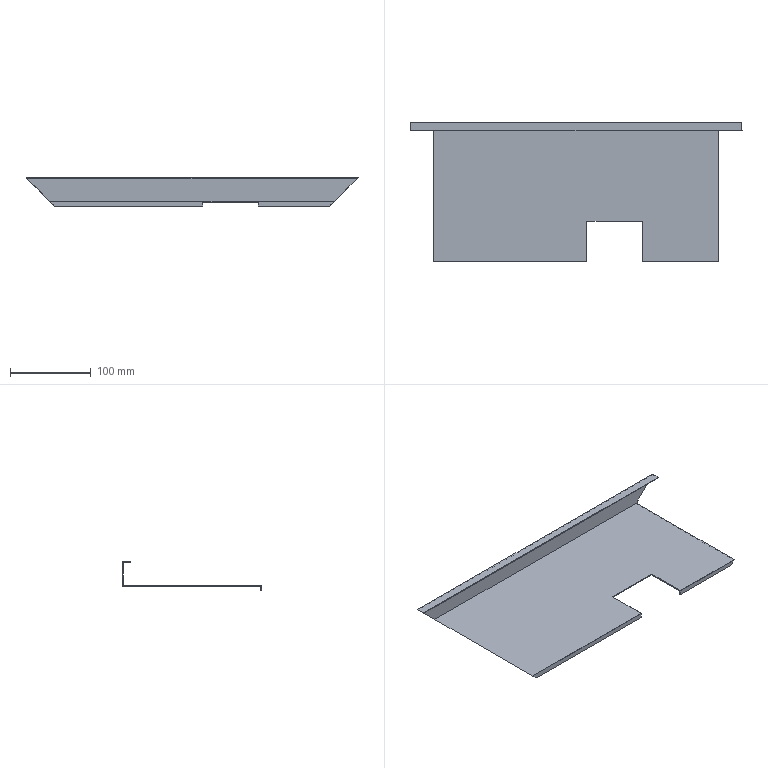Part | STEP file | 09-06 Inner side plate 3 | 1 solid | 18 faces | box 410 x 172 x 35 mm | volume 73059 mm3 | plane 18
STEP:
#1=CARTESIAN_POINT('',(0.,0.,0.));
#2=DIRECTION('',(0.,0.,1.));
#3=DIRECTION('',(1.,0.,0.));
#4=AXIS2_PLACEMENT_3D('',#1,#2,#3);
#5=CARTESIAN_POINT('',(381.,0.,1.));
#6=VERTEX_POINT('',#5);
#7=CARTESIAN_POINT('',(287.,0.,1.));
#8=VERTEX_POINT('',#7);
#9=CARTESIAN_POINT('',(205.,0.,1.));
#10=DIRECTION('',(-1.,0.,0.));
#11=VECTOR('',#10,1.);
#12=LINE('',#9,#11);
#13=CARTESIAN_POINT('',(29.,0.,1.));
#14=DIRECTION('',(0.,0.,-1.));
#15=DIRECTION('',(0.,1.,0.));
#16=AXIS2_PLACEMENT_3D('',#13,#14,#15);
#17=PLANE('',#16);
#18=CARTESIAN_POINT('',(0.,176.));
#19=DIRECTION('',(0.,-1.));
#20=VECTOR('',#19,1.);
#21=LINE('',#18,#20);
#22=(GEOMETRIC_REPRESENTATION_CONTEXT(2)PARAMETRIC_REPRESENTATION_CONTEXT()REPRESENTATION_CONTEXT('',''));
#23=DEFINITIONAL_REPRESENTATION('',(#21),#22);
#24=PCURVE('',#17,#23);
#25=CARTESIAN_POINT('',(287.,0.,-5.));
#26=DIRECTION('',(0.,1.,0.));
#27=DIRECTION('',(0.,0.,1.));
#28=AXIS2_PLACEMENT_3D('',#25,#26,#27);
#29=PLANE('',#28);
#30=CARTESIAN_POINT('',(6.,-82.));
#31=DIRECTION('',(0.,-1.));
#32=VECTOR('',#31,1.);
#33=LINE('',#30,#32);
#34=(GEOMETRIC_REPRESENTATION_CONTEXT(2)PARAMETRIC_REPRESENTATION_CONTEXT()REPRESENTATION_CONTEXT('',''));
#35=DEFINITIONAL_REPRESENTATION('',(#33),#34);
#36=PCURVE('',#29,#35);
#37=SURFACE_CURVE('',#12,(#24,#36),.PCURVE_S1.);
#38=EDGE_CURVE('',#6,#8,#37,.T.);
#39=ORIENTED_EDGE('',*,*,#38,.F.);
#40=CARTESIAN_POINT('',(381.,171.,1.));
#41=VERTEX_POINT('',#40);
#42=CARTESIAN_POINT('',(381.,85.5,1.));
#43=DIRECTION('',(0.,-1.,0.));
#44=VECTOR('',#43,1.);
#45=LINE('',#42,#44);
#46=CARTESIAN_POINT('',(85.5,352.));
#47=DIRECTION('',(-1.,0.));
#48=VECTOR('',#47,1.);
#49=LINE('',#46,#48);
#50=(GEOMETRIC_REPRESENTATION_CONTEXT(2)PARAMETRIC_REPRESENTATION_CONTEXT()REPRESENTATION_CONTEXT('',''));
#51=DEFINITIONAL_REPRESENTATION('',(#49),#50);
#52=PCURVE('',#17,#51);
#53=CARTESIAN_POINT('',(375.,0.,-5.));
#54=DIRECTION('',(-0.7071,0.,0.7071));
#55=DIRECTION('',(0.7071,0.,0.7071));
#56=AXIS2_PLACEMENT_3D('',#53,#54,#55);
#57=PLANE('',#56);
#58=CARTESIAN_POINT('',(8.485,85.5));
#59=DIRECTION('',(0.,-1.));
#60=VECTOR('',#59,1.);
#61=LINE('',#58,#60);
#62=(GEOMETRIC_REPRESENTATION_CONTEXT(2)PARAMETRIC_REPRESENTATION_CONTEXT()REPRESENTATION_CONTEXT('',''));
#63=DEFINITIONAL_REPRESENTATION('',(#61),#62);
#64=PCURVE('',#57,#63);
#65=SURFACE_CURVE('',#45,(#52,#64),.PCURVE_S1.);
#66=EDGE_CURVE('',#41,#6,#65,.T.);
#67=ORIENTED_EDGE('',*,*,#66,.F.);
#68=CARTESIAN_POINT('',(29.,171.,1.));
#69=VERTEX_POINT('',#68);
#70=CARTESIAN_POINT('',(205.,171.,1.));
#71=DIRECTION('',(1.,0.,0.));
#72=VECTOR('',#71,1.);
#73=LINE('',#70,#72);
#74=CARTESIAN_POINT('',(171.,176.));
#75=DIRECTION('',(0.,1.));
#76=VECTOR('',#75,1.);
#77=LINE('',#74,#76);
#78=(GEOMETRIC_REPRESENTATION_CONTEXT(2)PARAMETRIC_REPRESENTATION_CONTEXT()REPRESENTATION_CONTEXT('',''));
#79=DEFINITIONAL_REPRESENTATION('',(#77),#78);
#80=PCURVE('',#17,#79);
#81=CARTESIAN_POINT('',(-1.448,171.,1.));
#82=DIRECTION('',(0.,1.,0.));
#83=DIRECTION('',(0.,0.,1.));
#84=AXIS2_PLACEMENT_3D('',#81,#82,#83);
#85=PLANE('',#84);
#86=CARTESIAN_POINT('',(0.,206.448));
#87=DIRECTION('',(0.,1.));
#88=VECTOR('',#87,1.);
#89=LINE('',#86,#88);
#90=(GEOMETRIC_REPRESENTATION_CONTEXT(2)PARAMETRIC_REPRESENTATION_CONTEXT()REPRESENTATION_CONTEXT('',''));
#91=DEFINITIONAL_REPRESENTATION('',(#89),#90);
#92=PCURVE('',#85,#91);
#93=SURFACE_CURVE('',#73,(#80,#92),.PCURVE_S1.);
#94=EDGE_CURVE('',#69,#41,#93,.T.);
#95=ORIENTED_EDGE('',*,*,#94,.F.);
#96=CARTESIAN_POINT('',(29.,0.,1.));
#97=VERTEX_POINT('',#96);
#98=CARTESIAN_POINT('',(29.,85.5,1.));
#99=DIRECTION('',(0.,1.,0.));
#100=VECTOR('',#99,1.);
#101=LINE('',#98,#100);
#102=CARTESIAN_POINT('',(85.5,0.));
#103=DIRECTION('',(1.,0.));
#104=VECTOR('',#103,1.);
#105=LINE('',#102,#104);
#106=(GEOMETRIC_REPRESENTATION_CONTEXT(2)PARAMETRIC_REPRESENTATION_CONTEXT()REPRESENTATION_CONTEXT('',''));
#107=DEFINITIONAL_REPRESENTATION('',(#105),#106);
#108=PCURVE('',#17,#107);
#109=CARTESIAN_POINT('',(0.,0.,30.));
#110=DIRECTION('',(0.7071,0.,0.7071));
#111=DIRECTION('',(0.7071,0.,-0.7071));
#112=AXIS2_PLACEMENT_3D('',#109,#110,#111);
#113=PLANE('',#112);
#114=CARTESIAN_POINT('',(41.012,85.5));
#115=DIRECTION('',(0.,1.));
#116=VECTOR('',#115,1.);
#117=LINE('',#114,#116);
#118=(GEOMETRIC_REPRESENTATION_CONTEXT(2)PARAMETRIC_REPRESENTATION_CONTEXT()REPRESENTATION_CONTEXT('',''));
#119=DEFINITIONAL_REPRESENTATION('',(#117),#118);
#120=PCURVE('',#113,#119);
#121=SURFACE_CURVE('',#101,(#108,#120),.PCURVE_S1.);
#122=EDGE_CURVE('',#97,#69,#121,.T.);
#123=ORIENTED_EDGE('',*,*,#122,.F.);
#124=CARTESIAN_POINT('',(218.5,0.,1.));
#125=VERTEX_POINT('',#124);
#126=CARTESIAN_POINT('',(205.,0.,1.));
#127=DIRECTION('',(-1.,0.,0.));
#128=VECTOR('',#127,1.);
#129=LINE('',#126,#128);
#130=CARTESIAN_POINT('',(0.,176.));
#131=DIRECTION('',(0.,-1.));
#132=VECTOR('',#131,1.);
#133=LINE('',#130,#132);
#134=(GEOMETRIC_REPRESENTATION_CONTEXT(2)PARAMETRIC_REPRESENTATION_CONTEXT()REPRESENTATION_CONTEXT('',''));
#135=DEFINITIONAL_REPRESENTATION('',(#133),#134);
#136=PCURVE('',#17,#135);
#137=CARTESIAN_POINT('',(27.863,0.,-5.));
#138=DIRECTION('',(0.,1.,0.));
#139=DIRECTION('',(0.,0.,1.));
#140=AXIS2_PLACEMENT_3D('',#137,#138,#139);
#141=PLANE('',#140);
#142=CARTESIAN_POINT('',(6.,177.137));
#143=DIRECTION('',(0.,-1.));
#144=VECTOR('',#143,1.);
#145=LINE('',#142,#144);
#146=(GEOMETRIC_REPRESENTATION_CONTEXT(2)PARAMETRIC_REPRESENTATION_CONTEXT()REPRESENTATION_CONTEXT('',''));
#147=DEFINITIONAL_REPRESENTATION('',(#145),#146);
#148=PCURVE('',#141,#147);
#149=SURFACE_CURVE('',#129,(#136,#148),.PCURVE_S1.);
#150=EDGE_CURVE('',#125,#97,#149,.T.);
#151=ORIENTED_EDGE('',*,*,#150,.F.);
#152=CARTESIAN_POINT('',(218.5,50.,1.));
#153=VERTEX_POINT('',#152);
#154=CARTESIAN_POINT('',(218.5,85.5,1.));
#155=DIRECTION('',(0.,-1.,0.));
#156=VECTOR('',#155,1.);
#157=LINE('',#154,#156);
#158=CARTESIAN_POINT('',(85.5,189.5));
#159=DIRECTION('',(-1.,0.));
#160=VECTOR('',#159,1.);
#161=LINE('',#158,#160);
#162=(GEOMETRIC_REPRESENTATION_CONTEXT(2)PARAMETRIC_REPRESENTATION_CONTEXT()REPRESENTATION_CONTEXT('',''));
#163=DEFINITIONAL_REPRESENTATION('',(#161),#162);
#164=PCURVE('',#17,#163);
#165=CARTESIAN_POINT('',(218.5,0.,1.));
#166=DIRECTION('',(1.,0.,0.));
#167=DIRECTION('',(0.,0.,-1.));
#168=AXIS2_PLACEMENT_3D('',#165,#166,#167);
#169=PLANE('',#168);
#170=CARTESIAN_POINT('',(0.,85.5));
#171=DIRECTION('',(0.,-1.));
#172=VECTOR('',#171,1.);
#173=LINE('',#170,#172);
#174=(GEOMETRIC_REPRESENTATION_CONTEXT(2)PARAMETRIC_REPRESENTATION_CONTEXT()REPRESENTATION_CONTEXT('',''));
#175=DEFINITIONAL_REPRESENTATION('',(#173),#174);
#176=PCURVE('',#169,#175);
#177=SURFACE_CURVE('',#157,(#164,#176),.PCURVE_S1.);
#178=EDGE_CURVE('',#153,#125,#177,.T.);
#179=ORIENTED_EDGE('',*,*,#178,.F.);
#180=CARTESIAN_POINT('',(287.,50.,1.));
#181=VERTEX_POINT('',#180);
#182=CARTESIAN_POINT('',(205.,50.,1.));
#183=DIRECTION('',(-1.,0.,0.));
#184=VECTOR('',#183,1.);
#185=LINE('',#182,#184);
#186=CARTESIAN_POINT('',(50.,176.));
#187=DIRECTION('',(0.,-1.));
#188=VECTOR('',#187,1.);
#189=LINE('',#186,#188);
#190=(GEOMETRIC_REPRESENTATION_CONTEXT(2)PARAMETRIC_REPRESENTATION_CONTEXT()REPRESENTATION_CONTEXT('',''));
#191=DEFINITIONAL_REPRESENTATION('',(#189),#190);
#192=PCURVE('',#17,#191);
#193=CARTESIAN_POINT('',(218.5,50.,1.));
#194=DIRECTION('',(0.,-1.,0.));
#195=DIRECTION('',(0.,0.,-1.));
#196=AXIS2_PLACEMENT_3D('',#193,#194,#195);
#197=PLANE('',#196);
#198=CARTESIAN_POINT('',(0.,-13.5));
#199=DIRECTION('',(0.,-1.));
#200=VECTOR('',#199,1.);
#201=LINE('',#198,#200);
#202=(GEOMETRIC_REPRESENTATION_CONTEXT(2)PARAMETRIC_REPRESENTATION_CONTEXT()REPRESENTATION_CONTEXT('',''));
#203=DEFINITIONAL_REPRESENTATION('',(#201),#202);
#204=PCURVE('',#197,#203);
#205=SURFACE_CURVE('',#185,(#192,#204),.PCURVE_S1.);
#206=EDGE_CURVE('',#181,#153,#205,.T.);
#207=ORIENTED_EDGE('',*,*,#206,.F.);
#208=CARTESIAN_POINT('',(287.,85.5,1.));
#209=DIRECTION('',(0.,1.,0.));
#210=VECTOR('',#209,1.);
#211=LINE('',#208,#210);
#212=CARTESIAN_POINT('',(85.5,258.));
#213=DIRECTION('',(1.,0.));
#214=VECTOR('',#213,1.);
#215=LINE('',#212,#214);
#216=(GEOMETRIC_REPRESENTATION_CONTEXT(2)PARAMETRIC_REPRESENTATION_CONTEXT()REPRESENTATION_CONTEXT('',''));
#217=DEFINITIONAL_REPRESENTATION('',(#215),#216);
#218=PCURVE('',#17,#217);
#219=CARTESIAN_POINT('',(287.,0.,-5.));
#220=DIRECTION('',(-1.,0.,0.));
#221=DIRECTION('',(0.,0.,1.));
#222=AXIS2_PLACEMENT_3D('',#219,#220,#221);
#223=PLANE('',#222);
#224=CARTESIAN_POINT('',(6.,85.5));
#225=DIRECTION('',(0.,1.));
#226=VECTOR('',#225,1.);
#227=LINE('',#224,#226);
#228=(GEOMETRIC_REPRESENTATION_CONTEXT(2)PARAMETRIC_REPRESENTATION_CONTEXT()REPRESENTATION_CONTEXT('',''));
#229=DEFINITIONAL_REPRESENTATION('',(#227),#228);
#230=PCURVE('',#223,#229);
#231=SURFACE_CURVE('',#211,(#218,#230),.PCURVE_S1.);
#232=EDGE_CURVE('',#8,#181,#231,.T.);
#233=ORIENTED_EDGE('',*,*,#232,.F.);
#234=EDGE_LOOP('',(#39,#67,#95,#123,#151,#179,#207,#233));
#235=FACE_BOUND('',#234,.T.);
#236=ADVANCED_FACE('',(#235),#17,.F.);
#237=CARTESIAN_POINT('',(287.,1.,-5.));
#238=VERTEX_POINT('',#237);
#239=CARTESIAN_POINT('',(287.,0.,-5.));
#240=VERTEX_POINT('',#239);
#241=CARTESIAN_POINT('',(287.,0.5,-5.));
#242=DIRECTION('',(0.,-1.,0.));
#243=VECTOR('',#242,1.);
#244=LINE('',#241,#243);
#245=CARTESIAN_POINT('',(0.,0.5));
#246=DIRECTION('',(0.,-1.));
#247=VECTOR('',#246,1.);
#248=LINE('',#245,#247);
#249=(GEOMETRIC_REPRESENTATION_CONTEXT(2)PARAMETRIC_REPRESENTATION_CONTEXT()REPRESENTATION_CONTEXT('',''));
#250=DEFINITIONAL_REPRESENTATION('',(#248),#249);
#251=PCURVE('',#223,#250);
#252=CARTESIAN_POINT('',(287.,0.,-5.));
#253=DIRECTION('',(0.,0.,1.));
#254=DIRECTION('',(1.,0.,0.));
#255=AXIS2_PLACEMENT_3D('',#252,#253,#254);
#256=PLANE('',#255);
#257=CARTESIAN_POINT('',(0.,0.5));
#258=DIRECTION('',(0.,-1.));
#259=VECTOR('',#258,1.);
#260=LINE('',#257,#259);
#261=(GEOMETRIC_REPRESENTATION_CONTEXT(2)PARAMETRIC_REPRESENTATION_CONTEXT()REPRESENTATION_CONTEXT('',''));
#262=DEFINITIONAL_REPRESENTATION('',(#260),#261);
#263=PCURVE('',#256,#262);
#264=SURFACE_CURVE('',#244,(#251,#263),.PCURVE_S1.);
#265=EDGE_CURVE('',#238,#240,#264,.T.);
#266=ORIENTED_EDGE('',*,*,#265,.T.);
#267=CARTESIAN_POINT('',(287.,0.,-2.));
#268=DIRECTION('',(0.,0.,1.));
#269=VECTOR('',#268,1.);
#270=LINE('',#267,#269);
#271=CARTESIAN_POINT('',(3.,0.));
#272=DIRECTION('',(1.,0.));
#273=VECTOR('',#272,1.);
#274=LINE('',#271,#273);
#275=(GEOMETRIC_REPRESENTATION_CONTEXT(2)PARAMETRIC_REPRESENTATION_CONTEXT()REPRESENTATION_CONTEXT('',''));
#276=DEFINITIONAL_REPRESENTATION('',(#274),#275);
#277=PCURVE('',#223,#276);
#278=CARTESIAN_POINT('',(3.,0.));
#279=DIRECTION('',(1.,0.));
#280=VECTOR('',#279,1.);
#281=LINE('',#278,#280);
#282=(GEOMETRIC_REPRESENTATION_CONTEXT(2)PARAMETRIC_REPRESENTATION_CONTEXT()REPRESENTATION_CONTEXT('',''));
#283=DEFINITIONAL_REPRESENTATION('',(#281),#282);
#284=PCURVE('',#29,#283);
#285=SURFACE_CURVE('',#270,(#277,#284),.PCURVE_S1.);
#286=EDGE_CURVE('',#240,#8,#285,.T.);
#287=ORIENTED_EDGE('',*,*,#286,.T.);
#288=ORIENTED_EDGE('',*,*,#232,.T.);
#289=CARTESIAN_POINT('',(287.,50.,-0.000000001));
#290=VERTEX_POINT('',#289);
#291=CARTESIAN_POINT('',(287.,50.,-2.));
#292=DIRECTION('',(0.,0.,-1.));
#293=VECTOR('',#292,1.);
#294=LINE('',#291,#293);
#295=CARTESIAN_POINT('',(3.,50.));
#296=DIRECTION('',(-1.,0.));
#297=VECTOR('',#296,1.);
#298=LINE('',#295,#297);
#299=(GEOMETRIC_REPRESENTATION_CONTEXT(2)PARAMETRIC_REPRESENTATION_CONTEXT()REPRESENTATION_CONTEXT('',''));
#300=DEFINITIONAL_REPRESENTATION('',(#298),#299);
#301=PCURVE('',#223,#300);
#302=CARTESIAN_POINT('',(3.,68.5));
#303=DIRECTION('',(1.,0.));
#304=VECTOR('',#303,1.);
#305=LINE('',#302,#304);
#306=(GEOMETRIC_REPRESENTATION_CONTEXT(2)PARAMETRIC_REPRESENTATION_CONTEXT()REPRESENTATION_CONTEXT('',''));
#307=DEFINITIONAL_REPRESENTATION('',(#305),#306);
#308=PCURVE('',#197,#307);
#309=SURFACE_CURVE('',#294,(#301,#308),.PCURVE_S1.);
#310=EDGE_CURVE('',#181,#290,#309,.T.);
#311=ORIENTED_EDGE('',*,*,#310,.T.);
#312=CARTESIAN_POINT('',(287.,1.,-0.000000001));
#313=VERTEX_POINT('',#312);
#314=CARTESIAN_POINT('',(287.,25.,-0.000000002));
#315=DIRECTION('',(0.,-1.,0.));
#316=VECTOR('',#315,1.);
#317=LINE('',#314,#316);
#318=CARTESIAN_POINT('',(5.,25.));
#319=DIRECTION('',(0.,-1.));
#320=VECTOR('',#319,1.);
#321=LINE('',#318,#320);
#322=(GEOMETRIC_REPRESENTATION_CONTEXT(2)PARAMETRIC_REPRESENTATION_CONTEXT()REPRESENTATION_CONTEXT('',''));
#323=DEFINITIONAL_REPRESENTATION('',(#321),#322);
#324=PCURVE('',#223,#323);
#325=CARTESIAN_POINT('',(30.,172.,0.));
#326=DIRECTION('',(0.,0.,1.));
#327=DIRECTION('',(0.,-1.,0.));
#328=AXIS2_PLACEMENT_3D('',#325,#326,#327);
#329=PLANE('',#328);
#330=CARTESIAN_POINT('',(147.,257.));
#331=DIRECTION('',(1.,0.));
#332=VECTOR('',#331,1.);
#333=LINE('',#330,#332);
#334=(GEOMETRIC_REPRESENTATION_CONTEXT(2)PARAMETRIC_REPRESENTATION_CONTEXT()REPRESENTATION_CONTEXT('',''));
#335=DEFINITIONAL_REPRESENTATION('',(#333),#334);
#336=PCURVE('',#329,#335);
#337=SURFACE_CURVE('',#317,(#324,#336),.PCURVE_S1.);
#338=EDGE_CURVE('',#290,#313,#337,.T.);
#339=ORIENTED_EDGE('',*,*,#338,.T.);
#340=CARTESIAN_POINT('',(287.,1.,-2.));
#341=DIRECTION('',(0.,0.,-1.));
#342=VECTOR('',#341,1.);
#343=LINE('',#340,#342);
#344=CARTESIAN_POINT('',(3.,1.));
#345=DIRECTION('',(-1.,0.));
#346=VECTOR('',#345,1.);
#347=LINE('',#344,#346);
#348=(GEOMETRIC_REPRESENTATION_CONTEXT(2)PARAMETRIC_REPRESENTATION_CONTEXT()REPRESENTATION_CONTEXT('',''));
#349=DEFINITIONAL_REPRESENTATION('',(#347),#348);
#350=PCURVE('',#223,#349);
#351=CARTESIAN_POINT('',(287.,1.,0.));
#352=DIRECTION('',(0.,-1.,0.));
#353=DIRECTION('',(0.,0.,-1.));
#354=AXIS2_PLACEMENT_3D('',#351,#352,#353);
#355=PLANE('',#354);
#356=CARTESIAN_POINT('',(2.,0.));
#357=DIRECTION('',(1.,0.));
#358=VECTOR('',#357,1.);
#359=LINE('',#356,#358);
#360=(GEOMETRIC_REPRESENTATION_CONTEXT(2)PARAMETRIC_REPRESENTATION_CONTEXT()REPRESENTATION_CONTEXT('',''));
#361=DEFINITIONAL_REPRESENTATION('',(#359),#360);
#362=PCURVE('',#355,#361);
#363=SURFACE_CURVE('',#343,(#350,#362),.PCURVE_S1.);
#364=EDGE_CURVE('',#313,#238,#363,.T.);
#365=ORIENTED_EDGE('',*,*,#364,.T.);
#366=EDGE_LOOP('',(#266,#287,#288,#311,#339,#365));
#367=FACE_BOUND('',#366,.T.);
#368=ADVANCED_FACE('',(#367),#223,.T.);
#369=CARTESIAN_POINT('',(375.,0.,-5.));
#370=VERTEX_POINT('',#369);
#371=CARTESIAN_POINT('',(334.282,0.,-5.));
#372=DIRECTION('',(-1.,0.,0.));
#373=VECTOR('',#372,1.);
#374=LINE('',#371,#373);
#375=CARTESIAN_POINT('',(0.,47.282));
#376=DIRECTION('',(0.,-1.));
#377=VECTOR('',#376,1.);
#378=LINE('',#375,#377);
#379=(GEOMETRIC_REPRESENTATION_CONTEXT(2)PARAMETRIC_REPRESENTATION_CONTEXT()REPRESENTATION_CONTEXT('',''));
#380=DEFINITIONAL_REPRESENTATION('',(#378),#379);
#381=PCURVE('',#29,#380);
#382=CARTESIAN_POINT('',(47.282,0.));
#383=DIRECTION('',(-1.,0.));
#384=VECTOR('',#383,1.);
#385=LINE('',#382,#384);
#386=(GEOMETRIC_REPRESENTATION_CONTEXT(2)PARAMETRIC_REPRESENTATION_CONTEXT()REPRESENTATION_CONTEXT('',''));
#387=DEFINITIONAL_REPRESENTATION('',(#385),#386);
#388=PCURVE('',#256,#387);
#389=SURFACE_CURVE('',#374,(#381,#388),.PCURVE_S1.);
#390=EDGE_CURVE('',#370,#240,#389,.T.);
#391=ORIENTED_EDGE('',*,*,#390,.F.);
#392=CARTESIAN_POINT('',(375.,0.,-5.));
#393=DIRECTION('',(-0.7071,0.,-0.7071));
#394=VECTOR('',#393,1.);
#395=LINE('',#392,#394);
#396=CARTESIAN_POINT('',(0.,88.));
#397=DIRECTION('',(-0.7071,-0.7071));
#398=VECTOR('',#397,1.);
#399=LINE('',#396,#398);
#400=(GEOMETRIC_REPRESENTATION_CONTEXT(2)PARAMETRIC_REPRESENTATION_CONTEXT()REPRESENTATION_CONTEXT('',''));
#401=DEFINITIONAL_REPRESENTATION('',(#399),#400);
#402=PCURVE('',#29,#401);
#403=CARTESIAN_POINT('',(0.,0.));
#404=DIRECTION('',(-1.,0.));
#405=VECTOR('',#404,1.);
#406=LINE('',#403,#405);
#407=(GEOMETRIC_REPRESENTATION_CONTEXT(2)PARAMETRIC_REPRESENTATION_CONTEXT()REPRESENTATION_CONTEXT('',''));
#408=DEFINITIONAL_REPRESENTATION('',(#406),#407);
#409=PCURVE('',#57,#408);
#410=SURFACE_CURVE('',#395,(#402,#409),.PCURVE_S1.);
#411=EDGE_CURVE('',#6,#370,#410,.T.);
#412=ORIENTED_EDGE('',*,*,#411,.F.);
#413=ORIENTED_EDGE('',*,*,#38,.T.);
#414=ORIENTED_EDGE('',*,*,#286,.F.);
#415=EDGE_LOOP('',(#391,#412,#413,#414));
#416=FACE_BOUND('',#415,.T.);
#417=ADVANCED_FACE('',(#416),#29,.F.);
#418=CARTESIAN_POINT('',(410.,172.,30.));
#419=VERTEX_POINT('',#418);
#420=CARTESIAN_POINT('',(380.,172.,0.000000001));
#421=VERTEX_POINT('',#420);
#422=CARTESIAN_POINT('',(392.5,172.,12.5));
#423=DIRECTION('',(-0.7071,0.,-0.7071));
#424=VECTOR('',#423,1.);
#425=LINE('',#422,#424);
#426=CARTESIAN_POINT('',(24.749,172.));
#427=DIRECTION('',(-1.,0.));
#428=VECTOR('',#427,1.);
#429=LINE('',#426,#428);
#430=(GEOMETRIC_REPRESENTATION_CONTEXT(2)PARAMETRIC_REPRESENTATION_CONTEXT()REPRESENTATION_CONTEXT('',''));
#431=DEFINITIONAL_REPRESENTATION('',(#429),#430);
#432=PCURVE('',#57,#431);
#433=CARTESIAN_POINT('',(-2.46,172.,30.));
#434=DIRECTION('',(0.,-1.,0.));
#435=DIRECTION('',(0.,0.,-1.));
#436=AXIS2_PLACEMENT_3D('',#433,#434,#435);
#437=PLANE('',#436);
#438=CARTESIAN_POINT('',(17.5,394.96));
#439=DIRECTION('',(0.7071,-0.7071));
#440=VECTOR('',#439,1.);
#441=LINE('',#438,#440);
#442=(GEOMETRIC_REPRESENTATION_CONTEXT(2)PARAMETRIC_REPRESENTATION_CONTEXT()REPRESENTATION_CONTEXT('',''));
#443=DEFINITIONAL_REPRESENTATION('',(#441),#442);
#444=PCURVE('',#437,#443);
#445=SURFACE_CURVE('',#425,(#432,#444),.PCURVE_S1.);
#446=EDGE_CURVE('',#419,#421,#445,.T.);
#447=ORIENTED_EDGE('',*,*,#446,.F.);
#448=CARTESIAN_POINT('',(410.,162.,30.));
#449=VERTEX_POINT('',#448);
#450=CARTESIAN_POINT('',(410.,86.,30.));
#451=DIRECTION('',(0.,1.,0.));
#452=VECTOR('',#451,1.);
#453=LINE('',#450,#452);
#454=CARTESIAN_POINT('',(49.497,86.));
#455=DIRECTION('',(0.,1.));
#456=VECTOR('',#455,1.);
#457=LINE('',#454,#456);
#458=(GEOMETRIC_REPRESENTATION_CONTEXT(2)PARAMETRIC_REPRESENTATION_CONTEXT()REPRESENTATION_CONTEXT('',''));
#459=DEFINITIONAL_REPRESENTATION('',(#457),#458);
#460=PCURVE('',#57,#459);
#461=CARTESIAN_POINT('',(0.,162.,30.));
#462=DIRECTION('',(0.,0.,-1.));
#463=DIRECTION('',(0.,1.,0.));
#464=AXIS2_PLACEMENT_3D('',#461,#462,#463);
#465=PLANE('',#464);
#466=CARTESIAN_POINT('',(-76.,410.));
#467=DIRECTION('',(1.,0.));
#468=VECTOR('',#467,1.);
#469=LINE('',#466,#468);
#470=(GEOMETRIC_REPRESENTATION_CONTEXT(2)PARAMETRIC_REPRESENTATION_CONTEXT()REPRESENTATION_CONTEXT('',''));
#471=DEFINITIONAL_REPRESENTATION('',(#469),#470);
#472=PCURVE('',#465,#471);
#473=SURFACE_CURVE('',#453,(#460,#472),.PCURVE_S1.);
#474=EDGE_CURVE('',#449,#419,#473,.T.);
#475=ORIENTED_EDGE('',*,*,#474,.F.);
#476=CARTESIAN_POINT('',(409.,162.,29.));
#477=VERTEX_POINT('',#476);
#478=CARTESIAN_POINT('',(375.,162.,-5.));
#479=DIRECTION('',(-0.7071,0.,-0.7071));
#480=VECTOR('',#479,1.);
#481=LINE('',#478,#480);
#482=CARTESIAN_POINT('',(0.,162.));
#483=DIRECTION('',(-1.,0.));
#484=VECTOR('',#483,1.);
#485=LINE('',#482,#484);
#486=(GEOMETRIC_REPRESENTATION_CONTEXT(2)PARAMETRIC_REPRESENTATION_CONTEXT()REPRESENTATION_CONTEXT('',''));
#487=DEFINITIONAL_REPRESENTATION('',(#485),#486);
#488=PCURVE('',#57,#487);
#489=CARTESIAN_POINT('',(-2.46,162.,29.));
#490=DIRECTION('',(0.,1.,0.));
#491=DIRECTION('',(0.,0.,1.));
#492=AXIS2_PLACEMENT_3D('',#489,#490,#491);
#493=PLANE('',#492);
#494=CARTESIAN_POINT('',(-34.,377.46));
#495=DIRECTION('',(-0.7071,-0.7071));
#496=VECTOR('',#495,1.);
#497=LINE('',#494,#496);
#498=(GEOMETRIC_REPRESENTATION_CONTEXT(2)PARAMETRIC_REPRESENTATION_CONTEXT()REPRESENTATION_CONTEXT('',''));
#499=DEFINITIONAL_REPRESENTATION('',(#497),#498);
#500=PCURVE('',#493,#499);
#501=SURFACE_CURVE('',#481,(#488,#500),.PCURVE_S1.);
#502=EDGE_CURVE('',#449,#477,#501,.T.);
#503=ORIENTED_EDGE('',*,*,#502,.T.);
#504=CARTESIAN_POINT('',(409.,171.,29.));
#505=VERTEX_POINT('',#504);
#506=CARTESIAN_POINT('',(409.,86.,29.));
#507=DIRECTION('',(0.,-1.,0.));
#508=VECTOR('',#507,1.);
#509=LINE('',#506,#508);
#510=CARTESIAN_POINT('',(48.083,86.));
#511=DIRECTION('',(0.,-1.));
#512=VECTOR('',#511,1.);
#513=LINE('',#510,#512);
#514=(GEOMETRIC_REPRESENTATION_CONTEXT(2)PARAMETRIC_REPRESENTATION_CONTEXT()REPRESENTATION_CONTEXT('',''));
#515=DEFINITIONAL_REPRESENTATION('',(#513),#514);
#516=PCURVE('',#57,#515);
#517=CARTESIAN_POINT('',(1.,162.,29.));
#518=DIRECTION('',(0.,0.,1.));
#519=DIRECTION('',(1.,0.,0.));
#520=AXIS2_PLACEMENT_3D('',#517,#518,#519);
#521=PLANE('',#520);
#522=CARTESIAN_POINT('',(408.,-76.));
#523=DIRECTION('',(0.,-1.));
#524=VECTOR('',#523,1.);
#525=LINE('',#522,#524);
#526=(GEOMETRIC_REPRESENTATION_CONTEXT(2)PARAMETRIC_REPRESENTATION_CONTEXT()REPRESENTATION_CONTEXT('',''));
#527=DEFINITIONAL_REPRESENTATION('',(#525),#526);
#528=PCURVE('',#521,#527);
#529=SURFACE_CURVE('',#509,(#516,#528),.PCURVE_S1.);
#530=EDGE_CURVE('',#505,#477,#529,.T.);
#531=ORIENTED_EDGE('',*,*,#530,.F.);
#532=CARTESIAN_POINT('',(392.5,171.,12.5));
#533=DIRECTION('',(0.7071,0.,0.7071));
#534=VECTOR('',#533,1.);
#535=LINE('',#532,#534);
#536=CARTESIAN_POINT('',(24.749,171.));
#537=DIRECTION('',(1.,0.));
#538=VECTOR('',#537,1.);
#539=LINE('',#536,#538);
#540=(GEOMETRIC_REPRESENTATION_CONTEXT(2)PARAMETRIC_REPRESENTATION_CONTEXT()REPRESENTATION_CONTEXT('',''));
#541=DEFINITIONAL_REPRESENTATION('',(#539),#540);
#542=PCURVE('',#57,#541);
#543=CARTESIAN_POINT('',(11.5,393.948));
#544=DIRECTION('',(0.7071,0.7071));
#545=VECTOR('',#544,1.);
#546=LINE('',#543,#545);
#547=(GEOMETRIC_REPRESENTATION_CONTEXT(2)PARAMETRIC_REPRESENTATION_CONTEXT()REPRESENTATION_CONTEXT('',''));
#548=DEFINITIONAL_REPRESENTATION('',(#546),#547);
#549=PCURVE('',#85,#548);
#550=SURFACE_CURVE('',#535,(#542,#549),.PCURVE_S1.);
#551=EDGE_CURVE('',#41,#505,#550,.T.);
#552=ORIENTED_EDGE('',*,*,#551,.F.);
#553=ORIENTED_EDGE('',*,*,#66,.T.);
#554=ORIENTED_EDGE('',*,*,#411,.T.);
#555=CARTESIAN_POINT('',(375.,1.,-5.));
#556=VERTEX_POINT('',#555);
#557=CARTESIAN_POINT('',(375.,86.,-5.));
#558=DIRECTION('',(0.,-1.,0.));
#559=VECTOR('',#558,1.);
#560=LINE('',#557,#559);
#561=CARTESIAN_POINT('',(0.,86.));
#562=DIRECTION('',(0.,-1.));
#563=VECTOR('',#562,1.);
#564=LINE('',#561,#563);
#565=(GEOMETRIC_REPRESENTATION_CONTEXT(2)PARAMETRIC_REPRESENTATION_CONTEXT()REPRESENTATION_CONTEXT('',''));
#566=DEFINITIONAL_REPRESENTATION('',(#564),#565);
#567=PCURVE('',#57,#566);
#568=CARTESIAN_POINT('',(88.,86.));
#569=DIRECTION('',(0.,-1.));
#570=VECTOR('',#569,1.);
#571=LINE('',#568,#570);
#572=(GEOMETRIC_REPRESENTATION_CONTEXT(2)PARAMETRIC_REPRESENTATION_CONTEXT()REPRESENTATION_CONTEXT('',''));
#573=DEFINITIONAL_REPRESENTATION('',(#571),#572);
#574=PCURVE('',#256,#573);
#575=SURFACE_CURVE('',#560,(#567,#574),.PCURVE_S1.);
#576=EDGE_CURVE('',#556,#370,#575,.T.);
#577=ORIENTED_EDGE('',*,*,#576,.F.);
#578=CARTESIAN_POINT('',(380.,1.,0.000000001));
#579=VERTEX_POINT('',#578);
#580=CARTESIAN_POINT('',(392.5,1.,12.5));
#581=DIRECTION('',(-0.7071,0.,-0.7071));
#582=VECTOR('',#581,1.);
#583=LINE('',#580,#582);
#584=CARTESIAN_POINT('',(24.749,1.));
#585=DIRECTION('',(-1.,0.));
#586=VECTOR('',#585,1.);
#587=LINE('',#584,#586);
#588=(GEOMETRIC_REPRESENTATION_CONTEXT(2)PARAMETRIC_REPRESENTATION_CONTEXT()REPRESENTATION_CONTEXT('',''));
#589=DEFINITIONAL_REPRESENTATION('',(#587),#588);
#590=PCURVE('',#57,#589);
#591=CARTESIAN_POINT('',(-12.5,105.5));
#592=DIRECTION('',(0.7071,-0.7071));
#593=VECTOR('',#592,1.);
#594=LINE('',#591,#593);
#595=(GEOMETRIC_REPRESENTATION_CONTEXT(2)PARAMETRIC_REPRESENTATION_CONTEXT()REPRESENTATION_CONTEXT('',''));
#596=DEFINITIONAL_REPRESENTATION('',(#594),#595);
#597=PCURVE('',#355,#596);
#598=SURFACE_CURVE('',#583,(#590,#597),.PCURVE_S1.);
#599=EDGE_CURVE('',#579,#556,#598,.T.);
#600=ORIENTED_EDGE('',*,*,#599,.F.);
#601=CARTESIAN_POINT('',(380.,86.,0.000000005));
#602=DIRECTION('',(0.,-1.,0.));
#603=VECTOR('',#602,1.);
#604=LINE('',#601,#603);
#605=CARTESIAN_POINT('',(7.071,86.));
#606=DIRECTION('',(0.,-1.));
#607=VECTOR('',#606,1.);
#608=LINE('',#605,#607);
#609=(GEOMETRIC_REPRESENTATION_CONTEXT(2)PARAMETRIC_REPRESENTATION_CONTEXT()REPRESENTATION_CONTEXT('',''));
#610=DEFINITIONAL_REPRESENTATION('',(#608),#609);
#611=PCURVE('',#57,#610);
#612=CARTESIAN_POINT('',(86.,350.));
#613=DIRECTION('',(1.,0.));
#614=VECTOR('',#613,1.);
#615=LINE('',#612,#614);
#616=(GEOMETRIC_REPRESENTATION_CONTEXT(2)PARAMETRIC_REPRESENTATION_CONTEXT()REPRESENTATION_CONTEXT('',''));
#617=DEFINITIONAL_REPRESENTATION('',(#615),#616);
#618=PCURVE('',#329,#617);
#619=SURFACE_CURVE('',#604,(#611,#618),.PCURVE_S1.);
#620=EDGE_CURVE('',#421,#579,#619,.T.);
#621=ORIENTED_EDGE('',*,*,#620,.F.);
#622=EDGE_LOOP('',(#447,#475,#503,#531,#552,#553,#554,#577,#600,#621));
#623=FACE_BOUND('',#622,.T.);
#624=ADVANCED_FACE('',(#623),#57,.F.);
#625=ORIENTED_EDGE('',*,*,#551,.T.);
#626=CARTESIAN_POINT('',(1.,171.,29.));
#627=VERTEX_POINT('',#626);
#628=CARTESIAN_POINT('',(205.,171.,29.));
#629=DIRECTION('',(1.,0.,0.));
#630=VECTOR('',#629,1.);
#631=LINE('',#628,#630);
#632=CARTESIAN_POINT('',(28.,206.448));
#633=DIRECTION('',(0.,1.));
#634=VECTOR('',#633,1.);
#635=LINE('',#632,#634);
#636=(GEOMETRIC_REPRESENTATION_CONTEXT(2)PARAMETRIC_REPRESENTATION_CONTEXT()REPRESENTATION_CONTEXT('',''));
#637=DEFINITIONAL_REPRESENTATION('',(#635),#636);
#638=PCURVE('',#85,#637);
#639=CARTESIAN_POINT('',(204.,9.));
#640=DIRECTION('',(1.,0.));
#641=VECTOR('',#640,1.);
#642=LINE('',#639,#641);
#643=(GEOMETRIC_REPRESENTATION_CONTEXT(2)PARAMETRIC_REPRESENTATION_CONTEXT()REPRESENTATION_CONTEXT('',''));
#644=DEFINITIONAL_REPRESENTATION('',(#642),#643);
#645=PCURVE('',#521,#644);
#646=SURFACE_CURVE('',#631,(#638,#645),.PCURVE_S1.);
#647=EDGE_CURVE('',#627,#505,#646,.T.);
#648=ORIENTED_EDGE('',*,*,#647,.F.);
#649=CARTESIAN_POINT('',(0.,171.,30.));
#650=DIRECTION('',(-0.7071,0.,0.7071));
#651=VECTOR('',#650,1.);
#652=LINE('',#649,#651);
#653=CARTESIAN_POINT('',(29.,1.448));
#654=DIRECTION('',(0.7071,-0.7071));
#655=VECTOR('',#654,1.);
#656=LINE('',#653,#655);
#657=(GEOMETRIC_REPRESENTATION_CONTEXT(2)PARAMETRIC_REPRESENTATION_CONTEXT()REPRESENTATION_CONTEXT('',''));
#658=DEFINITIONAL_REPRESENTATION('',(#656),#657);
#659=PCURVE('',#85,#658);
#660=CARTESIAN_POINT('',(0.,171.));
#661=DIRECTION('',(-1.,0.));
#662=VECTOR('',#661,1.);
#663=LINE('',#660,#662);
#664=(GEOMETRIC_REPRESENTATION_CONTEXT(2)PARAMETRIC_REPRESENTATION_CONTEXT()REPRESENTATION_CONTEXT('',''));
#665=DEFINITIONAL_REPRESENTATION('',(#663),#664);
#666=PCURVE('',#113,#665);
#667=SURFACE_CURVE('',#652,(#659,#666),.PCURVE_S1.);
#668=EDGE_CURVE('',#69,#627,#667,.T.);
#669=ORIENTED_EDGE('',*,*,#668,.F.);
#670=ORIENTED_EDGE('',*,*,#94,.T.);
#671=EDGE_LOOP('',(#625,#648,#669,#670));
#672=FACE_BOUND('',#671,.T.);
#673=ADVANCED_FACE('',(#672),#85,.F.);
#674=CARTESIAN_POINT('',(35.,0.,-5.));
#675=VERTEX_POINT('',#674);
#676=CARTESIAN_POINT('',(17.5,0.,12.5));
#677=DIRECTION('',(0.7071,0.,-0.7071));
#678=VECTOR('',#677,1.);
#679=LINE('',#676,#678);
#680=CARTESIAN_POINT('',(24.749,0.));
#681=DIRECTION('',(1.,0.));
#682=VECTOR('',#681,1.);
#683=LINE('',#680,#682);
#684=(GEOMETRIC_REPRESENTATION_CONTEXT(2)PARAMETRIC_REPRESENTATION_CONTEXT()REPRESENTATION_CONTEXT('',''));
#685=DEFINITIONAL_REPRESENTATION('',(#683),#684);
#686=PCURVE('',#113,#685);
#687=CARTESIAN_POINT('',(17.5,-10.363));
#688=DIRECTION('',(-0.7071,0.7071));
#689=VECTOR('',#688,1.);
#690=LINE('',#687,#689);
#691=(GEOMETRIC_REPRESENTATION_CONTEXT(2)PARAMETRIC_REPRESENTATION_CONTEXT()REPRESENTATION_CONTEXT('',''));
#692=DEFINITIONAL_REPRESENTATION('',(#690),#691);
#693=PCURVE('',#141,#692);
#694=SURFACE_CURVE('',#679,(#686,#693),.PCURVE_S1.);
#695=EDGE_CURVE('',#97,#675,#694,.T.);
#696=ORIENTED_EDGE('',*,*,#695,.F.);
#697=ORIENTED_EDGE('',*,*,#122,.T.);
#698=ORIENTED_EDGE('',*,*,#668,.T.);
#699=CARTESIAN_POINT('',(1.,162.,29.));
#700=VERTEX_POINT('',#699);
#701=CARTESIAN_POINT('',(1.,86.,29.));
#702=DIRECTION('',(0.,1.,0.));
#703=VECTOR('',#702,1.);
#704=LINE('',#701,#703);
#705=CARTESIAN_POINT('',(1.414,86.));
#706=DIRECTION('',(0.,1.));
#707=VECTOR('',#706,1.);
#708=LINE('',#705,#707);
#709=(GEOMETRIC_REPRESENTATION_CONTEXT(2)PARAMETRIC_REPRESENTATION_CONTEXT()REPRESENTATION_CONTEXT('',''));
#710=DEFINITIONAL_REPRESENTATION('',(#708),#709);
#711=PCURVE('',#113,#710);
#712=CARTESIAN_POINT('',(0.000000015,-76.));
#713=DIRECTION('',(0.,1.));
#714=VECTOR('',#713,1.);
#715=LINE('',#712,#714);
#716=(GEOMETRIC_REPRESENTATION_CONTEXT(2)PARAMETRIC_REPRESENTATION_CONTEXT()REPRESENTATION_CONTEXT('',''));
#717=DEFINITIONAL_REPRESENTATION('',(#715),#716);
#718=PCURVE('',#521,#717);
#719=SURFACE_CURVE('',#704,(#711,#718),.PCURVE_S1.);
#720=EDGE_CURVE('',#700,#627,#719,.T.);
#721=ORIENTED_EDGE('',*,*,#720,.F.);
#722=CARTESIAN_POINT('',(0.,162.,30.));
#723=VERTEX_POINT('',#722);
#724=CARTESIAN_POINT('',(0.,162.,30.));
#725=DIRECTION('',(-0.7071,0.,0.7071));
#726=VECTOR('',#725,1.);
#727=LINE('',#724,#726);
#728=CARTESIAN_POINT('',(0.,162.));
#729=DIRECTION('',(-1.,0.));
#730=VECTOR('',#729,1.);
#731=LINE('',#728,#730);
#732=(GEOMETRIC_REPRESENTATION_CONTEXT(2)PARAMETRIC_REPRESENTATION_CONTEXT()REPRESENTATION_CONTEXT('',''));
#733=DEFINITIONAL_REPRESENTATION('',(#731),#732);
#734=PCURVE('',#113,#733);
#735=CARTESIAN_POINT('',(1.,2.46));
#736=DIRECTION('',(0.7071,-0.7071));
#737=VECTOR('',#736,1.);
#738=LINE('',#735,#737);
#739=(GEOMETRIC_REPRESENTATION_CONTEXT(2)PARAMETRIC_REPRESENTATION_CONTEXT()REPRESENTATION_CONTEXT('',''));
#740=DEFINITIONAL_REPRESENTATION('',(#738),#739);
#741=PCURVE('',#493,#740);
#742=SURFACE_CURVE('',#727,(#734,#741),.PCURVE_S1.);
#743=EDGE_CURVE('',#700,#723,#742,.T.);
#744=ORIENTED_EDGE('',*,*,#743,.T.);
#745=CARTESIAN_POINT('',(0.000000051,172.,30.));
#746=VERTEX_POINT('',#745);
#747=CARTESIAN_POINT('',(0.,86.,30.));
#748=DIRECTION('',(0.,-1.,0.));
#749=VECTOR('',#748,1.);
#750=LINE('',#747,#749);
#751=CARTESIAN_POINT('',(0.,86.));
#752=DIRECTION('',(0.,-1.));
#753=VECTOR('',#752,1.);
#754=LINE('',#751,#753);
#755=(GEOMETRIC_REPRESENTATION_CONTEXT(2)PARAMETRIC_REPRESENTATION_CONTEXT()REPRESENTATION_CONTEXT('',''));
#756=DEFINITIONAL_REPRESENTATION('',(#754),#755);
#757=PCURVE('',#113,#756);
#758=CARTESIAN_POINT('',(-76.,0.));
#759=DIRECTION('',(-1.,0.));
#760=VECTOR('',#759,1.);
#761=LINE('',#758,#760);
#762=(GEOMETRIC_REPRESENTATION_CONTEXT(2)PARAMETRIC_REPRESENTATION_CONTEXT()REPRESENTATION_CONTEXT('',''));
#763=DEFINITIONAL_REPRESENTATION('',(#761),#762);
#764=PCURVE('',#465,#763);
#765=SURFACE_CURVE('',#750,(#757,#764),.PCURVE_S1.);
#766=EDGE_CURVE('',#746,#723,#765,.T.);
#767=ORIENTED_EDGE('',*,*,#766,.F.);
#768=CARTESIAN_POINT('',(30.,172.,0.000000001));
#769=VERTEX_POINT('',#768);
#770=CARTESIAN_POINT('',(17.5,172.,12.5));
#771=DIRECTION('',(-0.7071,0.,0.7071));
#772=VECTOR('',#771,1.);
#773=LINE('',#770,#772);
#774=CARTESIAN_POINT('',(24.749,172.));
#775=DIRECTION('',(-1.,0.));
#776=VECTOR('',#775,1.);
#777=LINE('',#774,#776);
#778=(GEOMETRIC_REPRESENTATION_CONTEXT(2)PARAMETRIC_REPRESENTATION_CONTEXT()REPRESENTATION_CONTEXT('',''));
#779=DEFINITIONAL_REPRESENTATION('',(#777),#778);
#780=PCURVE('',#113,#779);
#781=CARTESIAN_POINT('',(17.5,19.96));
#782=DIRECTION('',(-0.7071,-0.7071));
#783=VECTOR('',#782,1.);
#784=LINE('',#781,#783);
#785=(GEOMETRIC_REPRESENTATION_CONTEXT(2)PARAMETRIC_REPRESENTATION_CONTEXT()REPRESENTATION_CONTEXT('',''));
#786=DEFINITIONAL_REPRESENTATION('',(#784),#785);
#787=PCURVE('',#437,#786);
#788=SURFACE_CURVE('',#773,(#780,#787),.PCURVE_S1.);
#789=EDGE_CURVE('',#769,#746,#788,.T.);
#790=ORIENTED_EDGE('',*,*,#789,.F.);
#791=CARTESIAN_POINT('',(30.,1.,0.000000001));
#792=VERTEX_POINT('',#791);
#793=CARTESIAN_POINT('',(30.,86.,0.000000005));
#794=DIRECTION('',(0.,1.,0.));
#795=VECTOR('',#794,1.);
#796=LINE('',#793,#795);
#797=CARTESIAN_POINT('',(42.426,86.));
#798=DIRECTION('',(0.,1.));
#799=VECTOR('',#798,1.);
#800=LINE('',#797,#799);
#801=(GEOMETRIC_REPRESENTATION_CONTEXT(2)PARAMETRIC_REPRESENTATION_CONTEXT()REPRESENTATION_CONTEXT('',''));
#802=DEFINITIONAL_REPRESENTATION('',(#800),#801);
#803=PCURVE('',#113,#802);
#804=CARTESIAN_POINT('',(86.,-0.000000005));
#805=DIRECTION('',(-1.,0.));
#806=VECTOR('',#805,1.);
#807=LINE('',#804,#806);
#808=(GEOMETRIC_REPRESENTATION_CONTEXT(2)PARAMETRIC_REPRESENTATION_CONTEXT()REPRESENTATION_CONTEXT('',''));
#809=DEFINITIONAL_REPRESENTATION('',(#807),#808);
#810=PCURVE('',#329,#809);
#811=SURFACE_CURVE('',#796,(#803,#810),.PCURVE_S1.);
#812=EDGE_CURVE('',#792,#769,#811,.T.);
#813=ORIENTED_EDGE('',*,*,#812,.F.);
#814=CARTESIAN_POINT('',(35.,1.,-5.));
#815=VERTEX_POINT('',#814);
#816=CARTESIAN_POINT('',(17.5,1.,12.5));
#817=DIRECTION('',(-0.7071,0.,0.7071));
#818=VECTOR('',#817,1.);
#819=LINE('',#816,#818);
#820=CARTESIAN_POINT('',(24.749,1.));
#821=DIRECTION('',(-1.,0.));
#822=VECTOR('',#821,1.);
#823=LINE('',#820,#822);
#824=(GEOMETRIC_REPRESENTATION_CONTEXT(2)PARAMETRIC_REPRESENTATION_CONTEXT()REPRESENTATION_CONTEXT('',''));
#825=DEFINITIONAL_REPRESENTATION('',(#823),#824);
#826=PCURVE('',#113,#825);
#827=CARTESIAN_POINT('',(28.869,1.,0.));
#828=DIRECTION('',(0.,-1.,0.));
#829=DIRECTION('',(0.,0.,-1.));
#830=AXIS2_PLACEMENT_3D('',#827,#828,#829);
#831=PLANE('',#830);
#832=CARTESIAN_POINT('',(-12.5,-11.369));
#833=DIRECTION('',(-0.7071,-0.7071));
#834=VECTOR('',#833,1.);
#835=LINE('',#832,#834);
#836=(GEOMETRIC_REPRESENTATION_CONTEXT(2)PARAMETRIC_REPRESENTATION_CONTEXT()REPRESENTATION_CONTEXT('',''));
#837=DEFINITIONAL_REPRESENTATION('',(#835),#836);
#838=PCURVE('',#831,#837);
#839=SURFACE_CURVE('',#819,(#826,#838),.PCURVE_S1.);
#840=EDGE_CURVE('',#815,#792,#839,.T.);
#841=ORIENTED_EDGE('',*,*,#840,.F.);
#842=CARTESIAN_POINT('',(35.,0.5,-5.));
#843=DIRECTION('',(0.,-1.,0.));
#844=VECTOR('',#843,1.);
#845=LINE('',#842,#844);
#846=CARTESIAN_POINT('',(49.497,0.5));
#847=DIRECTION('',(0.,-1.));
#848=VECTOR('',#847,1.);
#849=LINE('',#846,#848);
#850=(GEOMETRIC_REPRESENTATION_CONTEXT(2)PARAMETRIC_REPRESENTATION_CONTEXT()REPRESENTATION_CONTEXT('',''));
#851=DEFINITIONAL_REPRESENTATION('',(#849),#850);
#852=PCURVE('',#113,#851);
#853=CARTESIAN_POINT('',(35.,0.,-5.));
#854=DIRECTION('',(0.,0.,1.));
#855=DIRECTION('',(1.,0.,0.));
#856=AXIS2_PLACEMENT_3D('',#853,#854,#855);
#857=PLANE('',#856);
#858=CARTESIAN_POINT('',(0.,0.5));
#859=DIRECTION('',(0.,-1.));
#860=VECTOR('',#859,1.);
#861=LINE('',#858,#860);
#862=(GEOMETRIC_REPRESENTATION_CONTEXT(2)PARAMETRIC_REPRESENTATION_CONTEXT()REPRESENTATION_CONTEXT('',''));
#863=DEFINITIONAL_REPRESENTATION('',(#861),#862);
#864=PCURVE('',#857,#863);
#865=SURFACE_CURVE('',#845,(#852,#864),.PCURVE_S1.);
#866=EDGE_CURVE('',#815,#675,#865,.T.);
#867=ORIENTED_EDGE('',*,*,#866,.T.);
#868=EDGE_LOOP('',(#696,#697,#698,#721,#744,#767,#790,#813,#841,#867));
#869=FACE_BOUND('',#868,.T.);
#870=ADVANCED_FACE('',(#869),#113,.F.);
#871=ORIENTED_EDGE('',*,*,#150,.T.);
#872=ORIENTED_EDGE('',*,*,#695,.T.);
#873=CARTESIAN_POINT('',(218.5,0.,-5.));
#874=VERTEX_POINT('',#873);
#875=CARTESIAN_POINT('',(123.181,0.,-5.));
#876=DIRECTION('',(-1.,0.,0.));
#877=VECTOR('',#876,1.);
#878=LINE('',#875,#877);
#879=CARTESIAN_POINT('',(0.,95.319));
#880=DIRECTION('',(0.,-1.));
#881=VECTOR('',#880,1.);
#882=LINE('',#879,#881);
#883=(GEOMETRIC_REPRESENTATION_CONTEXT(2)PARAMETRIC_REPRESENTATION_CONTEXT()REPRESENTATION_CONTEXT('',''));
#884=DEFINITIONAL_REPRESENTATION('',(#882),#883);
#885=PCURVE('',#141,#884);
#886=CARTESIAN_POINT('',(88.181,0.));
#887=DIRECTION('',(-1.,0.));
#888=VECTOR('',#887,1.);
#889=LINE('',#886,#888);
#890=(GEOMETRIC_REPRESENTATION_CONTEXT(2)PARAMETRIC_REPRESENTATION_CONTEXT()REPRESENTATION_CONTEXT('',''));
#891=DEFINITIONAL_REPRESENTATION('',(#889),#890);
#892=PCURVE('',#857,#891);
#893=SURFACE_CURVE('',#878,(#885,#892),.PCURVE_S1.);
#894=EDGE_CURVE('',#874,#675,#893,.T.);
#895=ORIENTED_EDGE('',*,*,#894,.F.);
#896=CARTESIAN_POINT('',(218.5,0.,-2.));
#897=DIRECTION('',(0.,0.,-1.));
#898=VECTOR('',#897,1.);
#899=LINE('',#896,#898);
#900=CARTESIAN_POINT('',(3.,190.637));
#901=DIRECTION('',(-1.,0.));
#902=VECTOR('',#901,1.);
#903=LINE('',#900,#902);
#904=(GEOMETRIC_REPRESENTATION_CONTEXT(2)PARAMETRIC_REPRESENTATION_CONTEXT()REPRESENTATION_CONTEXT('',''));
#905=DEFINITIONAL_REPRESENTATION('',(#903),#904);
#906=PCURVE('',#141,#905);
#907=CARTESIAN_POINT('',(3.,0.));
#908=DIRECTION('',(1.,0.));
#909=VECTOR('',#908,1.);
#910=LINE('',#907,#909);
#911=(GEOMETRIC_REPRESENTATION_CONTEXT(2)PARAMETRIC_REPRESENTATION_CONTEXT()REPRESENTATION_CONTEXT('',''));
#912=DEFINITIONAL_REPRESENTATION('',(#910),#911);
#913=PCURVE('',#169,#912);
#914=SURFACE_CURVE('',#899,(#906,#913),.PCURVE_S1.);
#915=EDGE_CURVE('',#125,#874,#914,.T.);
#916=ORIENTED_EDGE('',*,*,#915,.F.);
#917=EDGE_LOOP('',(#871,#872,#895,#916));
#918=FACE_BOUND('',#917,.T.);
#919=ADVANCED_FACE('',(#918),#141,.F.);
#920=CARTESIAN_POINT('',(218.5,1.,-0.000000001));
#921=VERTEX_POINT('',#920);
#922=CARTESIAN_POINT('',(218.5,50.,-0.000000001));
#923=VERTEX_POINT('',#922);
#924=CARTESIAN_POINT('',(218.5,25.,-0.000000002));
#925=DIRECTION('',(0.,1.,0.));
#926=VECTOR('',#925,1.);
#927=LINE('',#924,#926);
#928=CARTESIAN_POINT('',(1.,25.));
#929=DIRECTION('',(0.,1.));
#930=VECTOR('',#929,1.);
#931=LINE('',#928,#930);
#932=(GEOMETRIC_REPRESENTATION_CONTEXT(2)PARAMETRIC_REPRESENTATION_CONTEXT()REPRESENTATION_CONTEXT('',''));
#933=DEFINITIONAL_REPRESENTATION('',(#931),#932);
#934=PCURVE('',#169,#933);
#935=CARTESIAN_POINT('',(147.,188.5));
#936=DIRECTION('',(-1.,0.));
#937=VECTOR('',#936,1.);
#938=LINE('',#935,#937);
#939=(GEOMETRIC_REPRESENTATION_CONTEXT(2)PARAMETRIC_REPRESENTATION_CONTEXT()REPRESENTATION_CONTEXT('',''));
#940=DEFINITIONAL_REPRESENTATION('',(#938),#939);
#941=PCURVE('',#329,#940);
#942=SURFACE_CURVE('',#927,(#934,#941),.PCURVE_S1.);
#943=EDGE_CURVE('',#921,#923,#942,.T.);
#944=ORIENTED_EDGE('',*,*,#943,.T.);
#945=CARTESIAN_POINT('',(218.5,50.,-2.));
#946=DIRECTION('',(0.,0.,1.));
#947=VECTOR('',#946,1.);
#948=LINE('',#945,#947);
#949=CARTESIAN_POINT('',(3.,50.));
#950=DIRECTION('',(-1.,0.));
#951=VECTOR('',#950,1.);
#952=LINE('',#949,#951);
#953=(GEOMETRIC_REPRESENTATION_CONTEXT(2)PARAMETRIC_REPRESENTATION_CONTEXT()REPRESENTATION_CONTEXT('',''));
#954=DEFINITIONAL_REPRESENTATION('',(#952),#953);
#955=PCURVE('',#169,#954);
#956=CARTESIAN_POINT('',(3.,0.));
#957=DIRECTION('',(-1.,0.));
#958=VECTOR('',#957,1.);
#959=LINE('',#956,#958);
#960=(GEOMETRIC_REPRESENTATION_CONTEXT(2)PARAMETRIC_REPRESENTATION_CONTEXT()REPRESENTATION_CONTEXT('',''));
#961=DEFINITIONAL_REPRESENTATION('',(#959),#960);
#962=PCURVE('',#197,#961);
#963=SURFACE_CURVE('',#948,(#955,#962),.PCURVE_S1.);
#964=EDGE_CURVE('',#923,#153,#963,.T.);
#965=ORIENTED_EDGE('',*,*,#964,.T.);
#966=ORIENTED_EDGE('',*,*,#178,.T.);
#967=ORIENTED_EDGE('',*,*,#915,.T.);
#968=CARTESIAN_POINT('',(218.5,1.,-5.));
#969=VERTEX_POINT('',#968);
#970=CARTESIAN_POINT('',(218.5,25.,-5.));
#971=DIRECTION('',(0.,1.,0.));
#972=VECTOR('',#971,1.);
#973=LINE('',#970,#972);
#974=CARTESIAN_POINT('',(6.,25.));
#975=DIRECTION('',(0.,1.));
#976=VECTOR('',#975,1.);
#977=LINE('',#974,#976);
#978=(GEOMETRIC_REPRESENTATION_CONTEXT(2)PARAMETRIC_REPRESENTATION_CONTEXT()REPRESENTATION_CONTEXT('',''));
#979=DEFINITIONAL_REPRESENTATION('',(#977),#978);
#980=PCURVE('',#169,#979);
#981=CARTESIAN_POINT('',(183.5,25.));
#982=DIRECTION('',(0.,1.));
#983=VECTOR('',#982,1.);
#984=LINE('',#981,#983);
#985=(GEOMETRIC_REPRESENTATION_CONTEXT(2)PARAMETRIC_REPRESENTATION_CONTEXT()REPRESENTATION_CONTEXT('',''));
#986=DEFINITIONAL_REPRESENTATION('',(#984),#985);
#987=PCURVE('',#857,#986);
#988=SURFACE_CURVE('',#973,(#980,#987),.PCURVE_S1.);
#989=EDGE_CURVE('',#874,#969,#988,.T.);
#990=ORIENTED_EDGE('',*,*,#989,.T.);
#991=CARTESIAN_POINT('',(218.5,1.,-2.));
#992=DIRECTION('',(0.,0.,1.));
#993=VECTOR('',#992,1.);
#994=LINE('',#991,#993);
#995=CARTESIAN_POINT('',(3.,1.));
#996=DIRECTION('',(-1.,0.));
#997=VECTOR('',#996,1.);
#998=LINE('',#995,#997);
#999=(GEOMETRIC_REPRESENTATION_CONTEXT(2)PARAMETRIC_REPRESENTATION_CONTEXT()REPRESENTATION_CONTEXT('',''));
#1000=DEFINITIONAL_REPRESENTATION('',(#998),#999);
#1001=PCURVE('',#169,#1000);
#1002=CARTESIAN_POINT('',(2.,189.631));
#1003=DIRECTION('',(-1.,0.));
#1004=VECTOR('',#1003,1.);
#1005=LINE('',#1002,#1004);
#1006=(GEOMETRIC_REPRESENTATION_CONTEXT(2)PARAMETRIC_REPRESENTATION_CONTEXT()REPRESENTATION_CONTEXT('',''));
#1007=DEFINITIONAL_REPRESENTATION('',(#1005),#1006);
#1008=PCURVE('',#831,#1007);
#1009=SURFACE_CURVE('',#994,(#1001,#1008),.PCURVE_S1.);
#1010=EDGE_CURVE('',#969,#921,#1009,.T.);
#1011=ORIENTED_EDGE('',*,*,#1010,.T.);
#1012=EDGE_LOOP('',(#944,#965,#966,#967,#990,#1011));
#1013=FACE_BOUND('',#1012,.T.);
#1014=ADVANCED_FACE('',(#1013),#169,.T.);
#1015=CARTESIAN_POINT('',(252.75,50.,0.));
#1016=DIRECTION('',(1.,0.,0.));
#1017=VECTOR('',#1016,1.);
#1018=LINE('',#1015,#1017);
#1019=CARTESIAN_POINT('',(1.,34.25));
#1020=DIRECTION('',(0.,1.));
#1021=VECTOR('',#1020,1.);
#1022=LINE('',#1019,#1021);
#1023=(GEOMETRIC_REPRESENTATION_CONTEXT(2)PARAMETRIC_REPRESENTATION_CONTEXT()REPRESENTATION_CONTEXT('',''));
#1024=DEFINITIONAL_REPRESENTATION('',(#1022),#1023);
#1025=PCURVE('',#197,#1024);
#1026=CARTESIAN_POINT('',(122.,222.75));
#1027=DIRECTION('',(0.,1.));
#1028=VECTOR('',#1027,1.);
#1029=LINE('',#1026,#1028);
#1030=(GEOMETRIC_REPRESENTATION_CONTEXT(2)PARAMETRIC_REPRESENTATION_CONTEXT()REPRESENTATION_CONTEXT('',''));
#1031=DEFINITIONAL_REPRESENTATION('',(#1029),#1030);
#1032=PCURVE('',#329,#1031);
#1033=SURFACE_CURVE('',#1018,(#1025,#1032),.PCURVE_S1.);
#1034=EDGE_CURVE('',#923,#290,#1033,.T.);
#1035=ORIENTED_EDGE('',*,*,#1034,.T.);
#1036=ORIENTED_EDGE('',*,*,#310,.F.);
#1037=ORIENTED_EDGE('',*,*,#206,.T.);
#1038=ORIENTED_EDGE('',*,*,#964,.F.);
#1039=EDGE_LOOP('',(#1035,#1036,#1037,#1038));
#1040=FACE_BOUND('',#1039,.T.);
#1041=ADVANCED_FACE('',(#1040),#197,.T.);
#1042=CARTESIAN_POINT('',(333.779,1.,0.));
#1043=DIRECTION('',(-1.,0.,0.));
#1044=VECTOR('',#1043,1.);
#1045=LINE('',#1042,#1044);
#1046=CARTESIAN_POINT('',(0.,46.779));
#1047=DIRECTION('',(0.,-1.));
#1048=VECTOR('',#1047,1.);
#1049=LINE('',#1046,#1048);
#1050=(GEOMETRIC_REPRESENTATION_CONTEXT(2)PARAMETRIC_REPRESENTATION_CONTEXT()REPRESENTATION_CONTEXT('',''));
#1051=DEFINITIONAL_REPRESENTATION('',(#1049),#1050);
#1052=PCURVE('',#355,#1051);
#1053=CARTESIAN_POINT('',(171.,303.779));
#1054=DIRECTION('',(0.,-1.));
#1055=VECTOR('',#1054,1.);
#1056=LINE('',#1053,#1055);
#1057=(GEOMETRIC_REPRESENTATION_CONTEXT(2)PARAMETRIC_REPRESENTATION_CONTEXT()REPRESENTATION_CONTEXT('',''));
#1058=DEFINITIONAL_REPRESENTATION('',(#1056),#1057);
#1059=PCURVE('',#329,#1058);
#1060=SURFACE_CURVE('',#1045,(#1052,#1059),.PCURVE_S1.);
#1061=EDGE_CURVE('',#579,#313,#1060,.T.);
#1062=ORIENTED_EDGE('',*,*,#1061,.F.);
#1063=ORIENTED_EDGE('',*,*,#599,.T.);
#1064=CARTESIAN_POINT('',(333.779,1.,-5.));
#1065=DIRECTION('',(1.,0.,0.));
#1066=VECTOR('',#1065,1.);
#1067=LINE('',#1064,#1066);
#1068=CARTESIAN_POINT('',(5.,46.779));
#1069=DIRECTION('',(0.,1.));
#1070=VECTOR('',#1069,1.);
#1071=LINE('',#1068,#1070);
#1072=(GEOMETRIC_REPRESENTATION_CONTEXT(2)PARAMETRIC_REPRESENTATION_CONTEXT()REPRESENTATION_CONTEXT('',''));
#1073=DEFINITIONAL_REPRESENTATION('',(#1071),#1072);
#1074=PCURVE('',#355,#1073);
#1075=CARTESIAN_POINT('',(46.779,1.));
#1076=DIRECTION('',(1.,0.));
#1077=VECTOR('',#1076,1.);
#1078=LINE('',#1075,#1077);
#1079=(GEOMETRIC_REPRESENTATION_CONTEXT(2)PARAMETRIC_REPRESENTATION_CONTEXT()REPRESENTATION_CONTEXT('',''));
#1080=DEFINITIONAL_REPRESENTATION('',(#1078),#1079);
#1081=PCURVE('',#256,#1080);
#1082=SURFACE_CURVE('',#1067,(#1074,#1081),.PCURVE_S1.);
#1083=EDGE_CURVE('',#238,#556,#1082,.T.);
#1084=ORIENTED_EDGE('',*,*,#1083,.F.);
#1085=ORIENTED_EDGE('',*,*,#364,.F.);
#1086=EDGE_LOOP('',(#1062,#1063,#1084,#1085));
#1087=FACE_BOUND('',#1086,.T.);
#1088=ADVANCED_FACE('',(#1087),#355,.F.);
#1089=ORIENTED_EDGE('',*,*,#1034,.F.);
#1090=ORIENTED_EDGE('',*,*,#943,.F.);
#1091=CARTESIAN_POINT('',(205.,1.,0.));
#1092=DIRECTION('',(1.,0.,0.));
#1093=VECTOR('',#1092,1.);
#1094=LINE('',#1091,#1093);
#1095=CARTESIAN_POINT('',(171.,175.));
#1096=DIRECTION('',(0.,1.));
#1097=VECTOR('',#1096,1.);
#1098=LINE('',#1095,#1097);
#1099=(GEOMETRIC_REPRESENTATION_CONTEXT(2)PARAMETRIC_REPRESENTATION_CONTEXT()REPRESENTATION_CONTEXT('',''));
#1100=DEFINITIONAL_REPRESENTATION('',(#1098),#1099);
#1101=PCURVE('',#329,#1100);
#1102=CARTESIAN_POINT('',(0.,176.131));
#1103=DIRECTION('',(0.,1.));
#1104=VECTOR('',#1103,1.);
#1105=LINE('',#1102,#1104);
#1106=(GEOMETRIC_REPRESENTATION_CONTEXT(2)PARAMETRIC_REPRESENTATION_CONTEXT()REPRESENTATION_CONTEXT('',''));
#1107=DEFINITIONAL_REPRESENTATION('',(#1105),#1106);
#1108=PCURVE('',#831,#1107);
#1109=SURFACE_CURVE('',#1094,(#1101,#1108),.PCURVE_S1.);
#1110=EDGE_CURVE('',#792,#921,#1109,.T.);
#1111=ORIENTED_EDGE('',*,*,#1110,.F.);
#1112=ORIENTED_EDGE('',*,*,#812,.T.);
#1113=CARTESIAN_POINT('',(205.,172.,0.));
#1114=DIRECTION('',(-1.,0.,0.));
#1115=VECTOR('',#1114,1.);
#1116=LINE('',#1113,#1115);
#1117=CARTESIAN_POINT('',(0.,175.));
#1118=DIRECTION('',(0.,-1.));
#1119=VECTOR('',#1118,1.);
#1120=LINE('',#1117,#1119);
#1121=(GEOMETRIC_REPRESENTATION_CONTEXT(2)PARAMETRIC_REPRESENTATION_CONTEXT()REPRESENTATION_CONTEXT('',''));
#1122=DEFINITIONAL_REPRESENTATION('',(#1120),#1121);
#1123=PCURVE('',#329,#1122);
#1124=CARTESIAN_POINT('',(30.,207.46));
#1125=DIRECTION('',(0.,-1.));
#1126=VECTOR('',#1125,1.);
#1127=LINE('',#1124,#1126);
#1128=(GEOMETRIC_REPRESENTATION_CONTEXT(2)PARAMETRIC_REPRESENTATION_CONTEXT()REPRESENTATION_CONTEXT('',''));
#1129=DEFINITIONAL_REPRESENTATION('',(#1127),#1128);
#1130=PCURVE('',#437,#1129);
#1131=SURFACE_CURVE('',#1116,(#1123,#1130),.PCURVE_S1.);
#1132=EDGE_CURVE('',#421,#769,#1131,.T.);
#1133=ORIENTED_EDGE('',*,*,#1132,.F.);
#1134=ORIENTED_EDGE('',*,*,#620,.T.);
#1135=ORIENTED_EDGE('',*,*,#1061,.T.);
#1136=ORIENTED_EDGE('',*,*,#338,.F.);
#1137=EDGE_LOOP('',(#1089,#1090,#1111,#1112,#1133,#1134,#1135,#1136));
#1138=FACE_BOUND('',#1137,.T.);
#1139=ADVANCED_FACE('',(#1138),#329,.F.);
#1140=ORIENTED_EDGE('',*,*,#1083,.T.);
#1141=ORIENTED_EDGE('',*,*,#576,.T.);
#1142=ORIENTED_EDGE('',*,*,#390,.T.);
#1143=ORIENTED_EDGE('',*,*,#265,.F.);
#1144=EDGE_LOOP('',(#1140,#1141,#1142,#1143));
#1145=FACE_BOUND('',#1144,.T.);
#1146=ADVANCED_FACE('',(#1145),#256,.F.);
#1147=ORIENTED_EDGE('',*,*,#446,.T.);
#1148=ORIENTED_EDGE('',*,*,#1132,.T.);
#1149=ORIENTED_EDGE('',*,*,#789,.T.);
#1150=CARTESIAN_POINT('',(205.,172.,30.));
#1151=DIRECTION('',(-1.,0.,0.));
#1152=VECTOR('',#1151,1.);
#1153=LINE('',#1150,#1152);
#1154=CARTESIAN_POINT('',(0.,207.46));
#1155=DIRECTION('',(0.,-1.));
#1156=VECTOR('',#1155,1.);
#1157=LINE('',#1154,#1156);
#1158=(GEOMETRIC_REPRESENTATION_CONTEXT(2)PARAMETRIC_REPRESENTATION_CONTEXT()REPRESENTATION_CONTEXT('',''));
#1159=DEFINITIONAL_REPRESENTATION('',(#1157),#1158);
#1160=PCURVE('',#437,#1159);
#1161=CARTESIAN_POINT('',(10.,205.));
#1162=DIRECTION('',(0.,-1.));
#1163=VECTOR('',#1162,1.);
#1164=LINE('',#1161,#1163);
#1165=(GEOMETRIC_REPRESENTATION_CONTEXT(2)PARAMETRIC_REPRESENTATION_CONTEXT()REPRESENTATION_CONTEXT('',''));
#1166=DEFINITIONAL_REPRESENTATION('',(#1164),#1165);
#1167=PCURVE('',#465,#1166);
#1168=SURFACE_CURVE('',#1153,(#1160,#1167),.PCURVE_S1.);
#1169=EDGE_CURVE('',#419,#746,#1168,.T.);
#1170=ORIENTED_EDGE('',*,*,#1169,.F.);
#1171=EDGE_LOOP('',(#1147,#1148,#1149,#1170));
#1172=FACE_BOUND('',#1171,.T.);
#1173=ADVANCED_FACE('',(#1172),#437,.F.);
#1174=CARTESIAN_POINT('',(205.,162.,30.));
#1175=DIRECTION('',(-1.,0.,0.));
#1176=VECTOR('',#1175,1.);
#1177=LINE('',#1174,#1176);
#1178=CARTESIAN_POINT('',(0.,205.));
#1179=DIRECTION('',(0.,-1.));
#1180=VECTOR('',#1179,1.);
#1181=LINE('',#1178,#1180);
#1182=(GEOMETRIC_REPRESENTATION_CONTEXT(2)PARAMETRIC_REPRESENTATION_CONTEXT()REPRESENTATION_CONTEXT('',''));
#1183=DEFINITIONAL_REPRESENTATION('',(#1181),#1182);
#1184=PCURVE('',#465,#1183);
#1185=CARTESIAN_POINT('',(1.,207.46));
#1186=DIRECTION('',(0.,-1.));
#1187=VECTOR('',#1186,1.);
#1188=LINE('',#1185,#1187);
#1189=(GEOMETRIC_REPRESENTATION_CONTEXT(2)PARAMETRIC_REPRESENTATION_CONTEXT()REPRESENTATION_CONTEXT('',''));
#1190=DEFINITIONAL_REPRESENTATION('',(#1188),#1189);
#1191=PCURVE('',#493,#1190);
#1192=SURFACE_CURVE('',#1177,(#1184,#1191),.PCURVE_S1.);
#1193=EDGE_CURVE('',#449,#723,#1192,.T.);
#1194=ORIENTED_EDGE('',*,*,#1193,.F.);
#1195=ORIENTED_EDGE('',*,*,#474,.T.);
#1196=ORIENTED_EDGE('',*,*,#1169,.T.);
#1197=ORIENTED_EDGE('',*,*,#766,.T.);
#1198=EDGE_LOOP('',(#1194,#1195,#1196,#1197));
#1199=FACE_BOUND('',#1198,.T.);
#1200=ADVANCED_FACE('',(#1199),#465,.F.);
#1201=ORIENTED_EDGE('',*,*,#530,.T.);
#1202=CARTESIAN_POINT('',(205.,162.,29.));
#1203=DIRECTION('',(1.,0.,0.));
#1204=VECTOR('',#1203,1.);
#1205=LINE('',#1202,#1204);
#1206=CARTESIAN_POINT('',(204.,0.));
#1207=DIRECTION('',(1.,0.));
#1208=VECTOR('',#1207,1.);
#1209=LINE('',#1206,#1208);
#1210=(GEOMETRIC_REPRESENTATION_CONTEXT(2)PARAMETRIC_REPRESENTATION_CONTEXT()REPRESENTATION_CONTEXT('',''));
#1211=DEFINITIONAL_REPRESENTATION('',(#1209),#1210);
#1212=PCURVE('',#521,#1211);
#1213=CARTESIAN_POINT('',(0.,207.46));
#1214=DIRECTION('',(0.,1.));
#1215=VECTOR('',#1214,1.);
#1216=LINE('',#1213,#1215);
#1217=(GEOMETRIC_REPRESENTATION_CONTEXT(2)PARAMETRIC_REPRESENTATION_CONTEXT()REPRESENTATION_CONTEXT('',''));
#1218=DEFINITIONAL_REPRESENTATION('',(#1216),#1217);
#1219=PCURVE('',#493,#1218);
#1220=SURFACE_CURVE('',#1205,(#1212,#1219),.PCURVE_S1.);
#1221=EDGE_CURVE('',#700,#477,#1220,.T.);
#1222=ORIENTED_EDGE('',*,*,#1221,.F.);
#1223=ORIENTED_EDGE('',*,*,#720,.T.);
#1224=ORIENTED_EDGE('',*,*,#647,.T.);
#1225=EDGE_LOOP('',(#1201,#1222,#1223,#1224));
#1226=FACE_BOUND('',#1225,.T.);
#1227=ADVANCED_FACE('',(#1226),#521,.F.);
#1228=CARTESIAN_POINT('',(123.684,1.,-5.));
#1229=DIRECTION('',(1.,0.,0.));
#1230=VECTOR('',#1229,1.);
#1231=LINE('',#1228,#1230);
#1232=CARTESIAN_POINT('',(5.,94.816));
#1233=DIRECTION('',(0.,1.));
#1234=VECTOR('',#1233,1.);
#1235=LINE('',#1232,#1234);
#1236=(GEOMETRIC_REPRESENTATION_CONTEXT(2)PARAMETRIC_REPRESENTATION_CONTEXT()REPRESENTATION_CONTEXT('',''));
#1237=DEFINITIONAL_REPRESENTATION('',(#1235),#1236);
#1238=PCURVE('',#831,#1237);
#1239=CARTESIAN_POINT('',(88.684,1.));
#1240=DIRECTION('',(1.,0.));
#1241=VECTOR('',#1240,1.);
#1242=LINE('',#1239,#1241);
#1243=(GEOMETRIC_REPRESENTATION_CONTEXT(2)PARAMETRIC_REPRESENTATION_CONTEXT()REPRESENTATION_CONTEXT('',''));
#1244=DEFINITIONAL_REPRESENTATION('',(#1242),#1243);
#1245=PCURVE('',#857,#1244);
#1246=SURFACE_CURVE('',#1231,(#1238,#1245),.PCURVE_S1.);
#1247=EDGE_CURVE('',#815,#969,#1246,.T.);
#1248=ORIENTED_EDGE('',*,*,#1247,.F.);
#1249=ORIENTED_EDGE('',*,*,#840,.T.);
#1250=ORIENTED_EDGE('',*,*,#1110,.T.);
#1251=ORIENTED_EDGE('',*,*,#1010,.F.);
#1252=EDGE_LOOP('',(#1248,#1249,#1250,#1251));
#1253=FACE_BOUND('',#1252,.T.);
#1254=ADVANCED_FACE('',(#1253),#831,.F.);
#1255=ORIENTED_EDGE('',*,*,#894,.T.);
#1256=ORIENTED_EDGE('',*,*,#866,.F.);
#1257=ORIENTED_EDGE('',*,*,#1247,.T.);
#1258=ORIENTED_EDGE('',*,*,#989,.F.);
#1259=EDGE_LOOP('',(#1255,#1256,#1257,#1258));
#1260=FACE_BOUND('',#1259,.T.);
#1261=ADVANCED_FACE('',(#1260),#857,.F.);
#1262=ORIENTED_EDGE('',*,*,#502,.F.);
#1263=ORIENTED_EDGE('',*,*,#1193,.T.);
#1264=ORIENTED_EDGE('',*,*,#743,.F.);
#1265=ORIENTED_EDGE('',*,*,#1221,.T.);
#1266=EDGE_LOOP('',(#1262,#1263,#1264,#1265));
#1267=FACE_BOUND('',#1266,.T.);
#1268=ADVANCED_FACE('',(#1267),#493,.F.);
#1269=CLOSED_SHELL('',(#236,#368,#417,#624,#673,#870,#919,#1014,#1041,#1088,#1139,#1146,#1173,#1200,#1227,#1254,#1261,#1268));
#1270=MANIFOLD_SOLID_BREP('',#1269);
#1271=(LENGTH_UNIT()NAMED_UNIT(*)SI_UNIT(.MILLI.,.METRE.));
#1272=UNCERTAINTY_MEASURE_WITH_UNIT(LENGTH_MEASURE(0.0000001),#1271,'','');
#1273=(NAMED_UNIT(*)PLANE_ANGLE_UNIT()SI_UNIT($,.RADIAN.));
#1274=(NAMED_UNIT(*)SI_UNIT($,.STERADIAN.)SOLID_ANGLE_UNIT());
#1275=(GEOMETRIC_REPRESENTATION_CONTEXT(3)GLOBAL_UNCERTAINTY_ASSIGNED_CONTEXT((#1272))GLOBAL_UNIT_ASSIGNED_CONTEXT((#1271,#1273,#1274))REPRESENTATION_CONTEXT('',''));
#1276=ADVANCED_BREP_SHAPE_REPRESENTATION('',(#4,#1270),#1275);